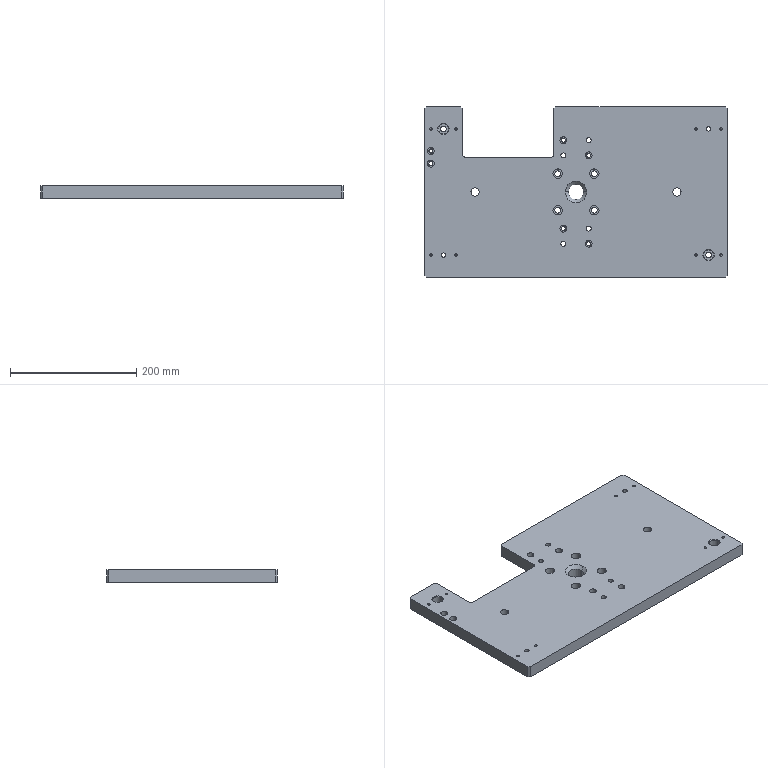Part | SolidWorks | features HoleWzd 9, Chamfer 3, Extrusion 1, Fillet 1 | 1 solid | 144 faces | box 480 x 270 x 20 mm | volume 2296067 mm3 | cylinder 88 | plane 30 | cone 26 | commonest cylinder face diameters 4.2 x16 6.6 x12 9 x12 11 x12 8 x8 15 x8